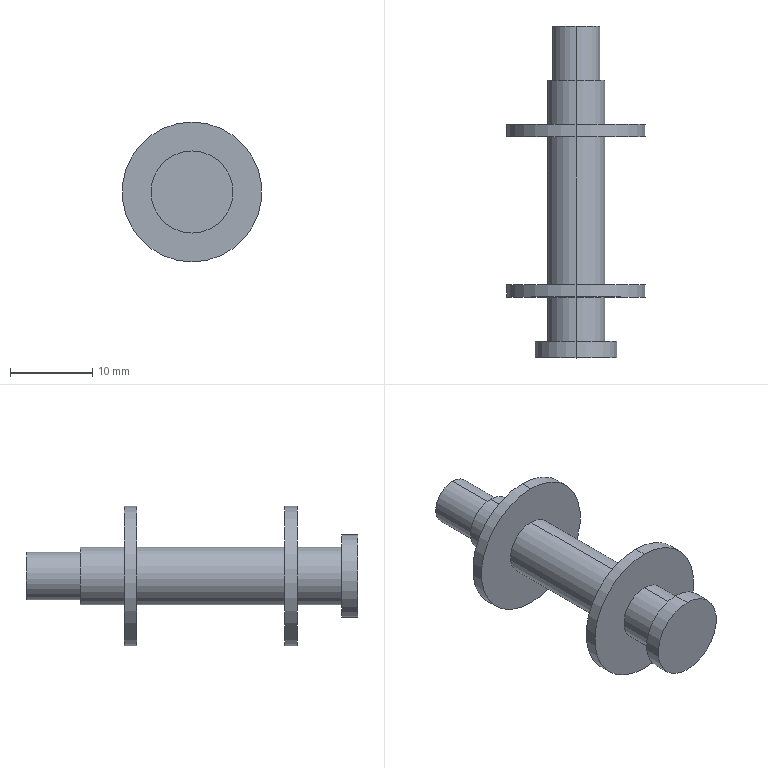Part | SolidWorks | features ICE 6, Extrusion 1 | 1 solid | 22 faces | box 17 x 40.37 x 17 mm | volume 2118 mm3 | cylinder 14 | plane 8 | commonest cylinder face diameters 7 x6 17 x4 5.77 x2 10 x2
STEP:
#1=CARTESIAN_POINT('',(0.,40.37,2.885));
#2=VERTEX_POINT('',#1);
#3=CARTESIAN_POINT('',(0.,40.37,-2.885));
#4=VERTEX_POINT('',#3);
#5=CARTESIAN_POINT('',(0.,40.37,0.));
#6=DIRECTION('',(0.,1.,0.));
#7=DIRECTION('',(0.,0.,1.));
#8=AXIS2_PLACEMENT_3D('',#5,#6,#7);
#9=CIRCLE('',#8,2.885);
#10=EDGE_CURVE('',#2,#4,#9,.T.);
#11=ORIENTED_EDGE('',*,*,#10,.F.);
#12=CARTESIAN_POINT('',(0.,33.8,2.885));
#13=VERTEX_POINT('',#12);
#14=CARTESIAN_POINT('',(0.,40.37,2.885));
#15=DIRECTION('',(0.,-1.,0.));
#16=VECTOR('',#15,1000.);
#17=LINE('',#14,#16);
#18=EDGE_CURVE('',#2,#13,#17,.T.);
#19=ORIENTED_EDGE('',*,*,#18,.T.);
#20=CARTESIAN_POINT('',(0.,33.8,-2.885));
#21=VERTEX_POINT('',#20);
#22=CARTESIAN_POINT('',(0.,33.8,0.));
#23=DIRECTION('',(0.,1.,0.));
#24=DIRECTION('',(0.,0.,1.));
#25=AXIS2_PLACEMENT_3D('',#22,#23,#24);
#26=CIRCLE('',#25,2.885);
#27=EDGE_CURVE('',#13,#21,#26,.T.);
#28=ORIENTED_EDGE('',*,*,#27,.T.);
#29=CARTESIAN_POINT('',(0.,40.37,-2.885));
#30=DIRECTION('',(0.,-1.,0.));
#31=VECTOR('',#30,1000.);
#32=LINE('',#29,#31);
#33=EDGE_CURVE('',#4,#21,#32,.T.);
#34=ORIENTED_EDGE('',*,*,#33,.F.);
#35=EDGE_LOOP('',(#11,#19,#28,#34));
#36=FACE_OUTER_BOUND('',#35,.T.);
#37=CARTESIAN_POINT('',(0.,40.37,0.));
#38=DIRECTION('',(0.,-1.,0.));
#39=DIRECTION('',(0.,0.,-1.));
#40=AXIS2_PLACEMENT_3D('',#37,#38,#39);
#41=CYLINDRICAL_SURFACE('',#40,2.885);
#42=ADVANCED_FACE('',(#36),#41,.T.);
#43=CARTESIAN_POINT('',(0.,33.8,3.5));
#44=VERTEX_POINT('',#43);
#45=CARTESIAN_POINT('',(0.,33.8,-3.5));
#46=VERTEX_POINT('',#45);
#47=CARTESIAN_POINT('',(0.,33.8,0.));
#48=DIRECTION('',(0.,1.,0.));
#49=DIRECTION('',(0.,0.,1.));
#50=AXIS2_PLACEMENT_3D('',#47,#48,#49);
#51=CIRCLE('',#50,3.5);
#52=EDGE_CURVE('',#44,#46,#51,.T.);
#53=ORIENTED_EDGE('',*,*,#52,.F.);
#54=CARTESIAN_POINT('',(0.,28.4,3.5));
#55=VERTEX_POINT('',#54);
#56=CARTESIAN_POINT('',(0.,33.8,3.5));
#57=DIRECTION('',(0.,-1.,0.));
#58=VECTOR('',#57,1000.);
#59=LINE('',#56,#58);
#60=EDGE_CURVE('',#44,#55,#59,.T.);
#61=ORIENTED_EDGE('',*,*,#60,.T.);
#62=CARTESIAN_POINT('',(0.,28.4,-3.5));
#63=VERTEX_POINT('',#62);
#64=CARTESIAN_POINT('',(0.,28.4,0.));
#65=DIRECTION('',(0.,1.,0.));
#66=DIRECTION('',(0.,0.,1.));
#67=AXIS2_PLACEMENT_3D('',#64,#65,#66);
#68=CIRCLE('',#67,3.5);
#69=EDGE_CURVE('',#55,#63,#68,.T.);
#70=ORIENTED_EDGE('',*,*,#69,.T.);
#71=CARTESIAN_POINT('',(0.,33.8,-3.5));
#72=DIRECTION('',(0.,-1.,0.));
#73=VECTOR('',#72,1000.);
#74=LINE('',#71,#73);
#75=EDGE_CURVE('',#46,#63,#74,.T.);
#76=ORIENTED_EDGE('',*,*,#75,.F.);
#77=EDGE_LOOP('',(#53,#61,#70,#76));
#78=FACE_OUTER_BOUND('',#77,.T.);
#79=CARTESIAN_POINT('',(0.,33.8,0.));
#80=DIRECTION('',(0.,-1.,0.));
#81=DIRECTION('',(0.,0.,-1.));
#82=AXIS2_PLACEMENT_3D('',#79,#80,#81);
#83=CYLINDRICAL_SURFACE('',#82,3.5);
#84=ADVANCED_FACE('',(#78),#83,.T.);
#85=CARTESIAN_POINT('',(0.,28.4,8.5));
#86=VERTEX_POINT('',#85);
#87=CARTESIAN_POINT('',(0.,28.4,-8.5));
#88=VERTEX_POINT('',#87);
#89=CARTESIAN_POINT('',(0.,28.4,0.));
#90=DIRECTION('',(0.,1.,0.));
#91=DIRECTION('',(0.,0.,1.));
#92=AXIS2_PLACEMENT_3D('',#89,#90,#91);
#93=CIRCLE('',#92,8.5);
#94=EDGE_CURVE('',#86,#88,#93,.T.);
#95=ORIENTED_EDGE('',*,*,#94,.F.);
#96=CARTESIAN_POINT('',(0.,26.9,8.5));
#97=VERTEX_POINT('',#96);
#98=CARTESIAN_POINT('',(0.,28.4,8.5));
#99=DIRECTION('',(0.,-1.,0.));
#100=VECTOR('',#99,1000.);
#101=LINE('',#98,#100);
#102=EDGE_CURVE('',#86,#97,#101,.T.);
#103=ORIENTED_EDGE('',*,*,#102,.T.);
#104=CARTESIAN_POINT('',(0.,26.9,-8.5));
#105=VERTEX_POINT('',#104);
#106=CARTESIAN_POINT('',(0.,26.9,0.));
#107=DIRECTION('',(0.,1.,0.));
#108=DIRECTION('',(0.,0.,1.));
#109=AXIS2_PLACEMENT_3D('',#106,#107,#108);
#110=CIRCLE('',#109,8.5);
#111=EDGE_CURVE('',#97,#105,#110,.T.);
#112=ORIENTED_EDGE('',*,*,#111,.T.);
#113=CARTESIAN_POINT('',(0.,28.4,-8.5));
#114=DIRECTION('',(0.,-1.,0.));
#115=VECTOR('',#114,1000.);
#116=LINE('',#113,#115);
#117=EDGE_CURVE('',#88,#105,#116,.T.);
#118=ORIENTED_EDGE('',*,*,#117,.F.);
#119=EDGE_LOOP('',(#95,#103,#112,#118));
#120=FACE_OUTER_BOUND('',#119,.T.);
#121=CARTESIAN_POINT('',(0.,28.4,0.));
#122=DIRECTION('',(0.,-1.,0.));
#123=DIRECTION('',(0.,0.,-1.));
#124=AXIS2_PLACEMENT_3D('',#121,#122,#123);
#125=CYLINDRICAL_SURFACE('',#124,8.5);
#126=ADVANCED_FACE('',(#120),#125,.T.);
#127=CARTESIAN_POINT('',(0.,26.9,3.5));
#128=VERTEX_POINT('',#127);
#129=CARTESIAN_POINT('',(0.,26.9,-3.5));
#130=VERTEX_POINT('',#129);
#131=CARTESIAN_POINT('',(0.,26.9,0.));
#132=DIRECTION('',(0.,1.,0.));
#133=DIRECTION('',(0.,0.,1.));
#134=AXIS2_PLACEMENT_3D('',#131,#132,#133);
#135=CIRCLE('',#134,3.5);
#136=EDGE_CURVE('',#128,#130,#135,.T.);
#137=ORIENTED_EDGE('',*,*,#136,.F.);
#138=CARTESIAN_POINT('',(0.,8.9,3.5));
#139=VERTEX_POINT('',#138);
#140=CARTESIAN_POINT('',(0.,26.9,3.5));
#141=DIRECTION('',(0.,-1.,0.));
#142=VECTOR('',#141,1000.);
#143=LINE('',#140,#142);
#144=EDGE_CURVE('',#128,#139,#143,.T.);
#145=ORIENTED_EDGE('',*,*,#144,.T.);
#146=CARTESIAN_POINT('',(0.,8.9,-3.5));
#147=VERTEX_POINT('',#146);
#148=CARTESIAN_POINT('',(0.,8.9,0.));
#149=DIRECTION('',(0.,1.,0.));
#150=DIRECTION('',(0.,0.,1.));
#151=AXIS2_PLACEMENT_3D('',#148,#149,#150);
#152=CIRCLE('',#151,3.5);
#153=EDGE_CURVE('',#139,#147,#152,.T.);
#154=ORIENTED_EDGE('',*,*,#153,.T.);
#155=CARTESIAN_POINT('',(0.,26.9,-3.5));
#156=DIRECTION('',(0.,-1.,0.));
#157=VECTOR('',#156,1000.);
#158=LINE('',#155,#157);
#159=EDGE_CURVE('',#130,#147,#158,.T.);
#160=ORIENTED_EDGE('',*,*,#159,.F.);
#161=EDGE_LOOP('',(#137,#145,#154,#160));
#162=FACE_OUTER_BOUND('',#161,.T.);
#163=CARTESIAN_POINT('',(0.,26.9,0.));
#164=DIRECTION('',(0.,-1.,0.));
#165=DIRECTION('',(0.,0.,-1.));
#166=AXIS2_PLACEMENT_3D('',#163,#164,#165);
#167=CYLINDRICAL_SURFACE('',#166,3.5);
#168=ADVANCED_FACE('',(#162),#167,.T.);
#169=CARTESIAN_POINT('',(0.,8.9,8.5));
#170=VERTEX_POINT('',#169);
#171=CARTESIAN_POINT('',(0.,8.9,-8.5));
#172=VERTEX_POINT('',#171);
#173=CARTESIAN_POINT('',(0.,8.9,0.));
#174=DIRECTION('',(0.,1.,0.));
#175=DIRECTION('',(0.,0.,1.));
#176=AXIS2_PLACEMENT_3D('',#173,#174,#175);
#177=CIRCLE('',#176,8.5);
#178=EDGE_CURVE('',#170,#172,#177,.T.);
#179=ORIENTED_EDGE('',*,*,#178,.F.);
#180=CARTESIAN_POINT('',(0.,7.4,8.5));
#181=VERTEX_POINT('',#180);
#182=CARTESIAN_POINT('',(0.,8.9,8.5));
#183=DIRECTION('',(0.,-1.,0.));
#184=VECTOR('',#183,1000.);
#185=LINE('',#182,#184);
#186=EDGE_CURVE('',#170,#181,#185,.T.);
#187=ORIENTED_EDGE('',*,*,#186,.T.);
#188=CARTESIAN_POINT('',(0.,7.4,-8.5));
#189=VERTEX_POINT('',#188);
#190=CARTESIAN_POINT('',(0.,7.4,0.));
#191=DIRECTION('',(0.,1.,0.));
#192=DIRECTION('',(0.,0.,1.));
#193=AXIS2_PLACEMENT_3D('',#190,#191,#192);
#194=CIRCLE('',#193,8.5);
#195=EDGE_CURVE('',#181,#189,#194,.T.);
#196=ORIENTED_EDGE('',*,*,#195,.T.);
#197=CARTESIAN_POINT('',(0.,8.9,-8.5));
#198=DIRECTION('',(0.,-1.,0.));
#199=VECTOR('',#198,1000.);
#200=LINE('',#197,#199);
#201=EDGE_CURVE('',#172,#189,#200,.T.);
#202=ORIENTED_EDGE('',*,*,#201,.F.);
#203=EDGE_LOOP('',(#179,#187,#196,#202));
#204=FACE_OUTER_BOUND('',#203,.T.);
#205=CARTESIAN_POINT('',(0.,8.9,0.));
#206=DIRECTION('',(0.,-1.,0.));
#207=DIRECTION('',(0.,0.,-1.));
#208=AXIS2_PLACEMENT_3D('',#205,#206,#207);
#209=CYLINDRICAL_SURFACE('',#208,8.5);
#210=ADVANCED_FACE('',(#204),#209,.T.);
#211=CARTESIAN_POINT('',(0.,7.4,3.5));
#212=VERTEX_POINT('',#211);
#213=CARTESIAN_POINT('',(0.,7.4,-3.5));
#214=VERTEX_POINT('',#213);
#215=CARTESIAN_POINT('',(0.,7.4,0.));
#216=DIRECTION('',(0.,1.,0.));
#217=DIRECTION('',(0.,0.,1.));
#218=AXIS2_PLACEMENT_3D('',#215,#216,#217);
#219=CIRCLE('',#218,3.5);
#220=EDGE_CURVE('',#212,#214,#219,.T.);
#221=ORIENTED_EDGE('',*,*,#220,.F.);
#222=CARTESIAN_POINT('',(0.,2.,3.5));
#223=VERTEX_POINT('',#222);
#224=CARTESIAN_POINT('',(0.,7.4,3.5));
#225=DIRECTION('',(0.,-1.,0.));
#226=VECTOR('',#225,1000.);
#227=LINE('',#224,#226);
#228=EDGE_CURVE('',#212,#223,#227,.T.);
#229=ORIENTED_EDGE('',*,*,#228,.T.);
#230=CARTESIAN_POINT('',(0.,2.,-3.5));
#231=VERTEX_POINT('',#230);
#232=CARTESIAN_POINT('',(0.,2.,0.));
#233=DIRECTION('',(0.,1.,0.));
#234=DIRECTION('',(0.,0.,1.));
#235=AXIS2_PLACEMENT_3D('',#232,#233,#234);
#236=CIRCLE('',#235,3.5);
#237=EDGE_CURVE('',#223,#231,#236,.T.);
#238=ORIENTED_EDGE('',*,*,#237,.T.);
#239=CARTESIAN_POINT('',(0.,7.4,-3.5));
#240=DIRECTION('',(0.,-1.,0.));
#241=VECTOR('',#240,1000.);
#242=LINE('',#239,#241);
#243=EDGE_CURVE('',#214,#231,#242,.T.);
#244=ORIENTED_EDGE('',*,*,#243,.F.);
#245=EDGE_LOOP('',(#221,#229,#238,#244));
#246=FACE_OUTER_BOUND('',#245,.T.);
#247=CARTESIAN_POINT('',(0.,7.4,0.));
#248=DIRECTION('',(0.,-1.,0.));
#249=DIRECTION('',(0.,0.,-1.));
#250=AXIS2_PLACEMENT_3D('',#247,#248,#249);
#251=CYLINDRICAL_SURFACE('',#250,3.5);
#252=ADVANCED_FACE('',(#246),#251,.T.);
#253=CARTESIAN_POINT('',(0.,2.,5.));
#254=VERTEX_POINT('',#253);
#255=CARTESIAN_POINT('',(0.,2.,-5.));
#256=VERTEX_POINT('',#255);
#257=CARTESIAN_POINT('',(0.,2.,0.));
#258=DIRECTION('',(0.,1.,0.));
#259=DIRECTION('',(0.,0.,1.));
#260=AXIS2_PLACEMENT_3D('',#257,#258,#259);
#261=CIRCLE('',#260,5.);
#262=EDGE_CURVE('',#254,#256,#261,.T.);
#263=ORIENTED_EDGE('',*,*,#262,.F.);
#264=CARTESIAN_POINT('',(0.,0.,5.));
#265=VERTEX_POINT('',#264);
#266=CARTESIAN_POINT('',(0.,2.,5.));
#267=DIRECTION('',(0.,-1.,0.));
#268=VECTOR('',#267,1000.);
#269=LINE('',#266,#268);
#270=EDGE_CURVE('',#254,#265,#269,.T.);
#271=ORIENTED_EDGE('',*,*,#270,.T.);
#272=CARTESIAN_POINT('',(0.,0.,-5.));
#273=VERTEX_POINT('',#272);
#274=CARTESIAN_POINT('',(0.,0.,0.));
#275=DIRECTION('',(0.,1.,0.));
#276=DIRECTION('',(0.,0.,1.));
#277=AXIS2_PLACEMENT_3D('',#274,#275,#276);
#278=CIRCLE('',#277,5.);
#279=EDGE_CURVE('',#265,#273,#278,.T.);
#280=ORIENTED_EDGE('',*,*,#279,.T.);
#281=CARTESIAN_POINT('',(0.,2.,-5.));
#282=DIRECTION('',(0.,-1.,0.));
#283=VECTOR('',#282,1000.);
#284=LINE('',#281,#283);
#285=EDGE_CURVE('',#256,#273,#284,.T.);
#286=ORIENTED_EDGE('',*,*,#285,.F.);
#287=EDGE_LOOP('',(#263,#271,#280,#286));
#288=FACE_OUTER_BOUND('',#287,.T.);
#289=CARTESIAN_POINT('',(0.,2.,0.));
#290=DIRECTION('',(0.,-1.,0.));
#291=DIRECTION('',(0.,0.,-1.));
#292=AXIS2_PLACEMENT_3D('',#289,#290,#291);
#293=CYLINDRICAL_SURFACE('',#292,5.);
#294=ADVANCED_FACE('',(#288),#293,.T.);
#295=ORIENTED_EDGE('',*,*,#270,.F.);
#296=CARTESIAN_POINT('',(0.,2.,0.));
#297=DIRECTION('',(0.,1.,0.));
#298=DIRECTION('',(0.,0.,1.));
#299=AXIS2_PLACEMENT_3D('',#296,#297,#298);
#300=CIRCLE('',#299,5.);
#301=EDGE_CURVE('',#256,#254,#300,.T.);
#302=ORIENTED_EDGE('',*,*,#301,.F.);
#303=ORIENTED_EDGE('',*,*,#285,.T.);
#304=CARTESIAN_POINT('',(0.,0.,0.));
#305=DIRECTION('',(0.,1.,0.));
#306=DIRECTION('',(0.,0.,1.));
#307=AXIS2_PLACEMENT_3D('',#304,#305,#306);
#308=CIRCLE('',#307,5.);
#309=EDGE_CURVE('',#273,#265,#308,.T.);
#310=ORIENTED_EDGE('',*,*,#309,.T.);
#311=EDGE_LOOP('',(#295,#302,#303,#310));
#312=FACE_OUTER_BOUND('',#311,.T.);
#313=CARTESIAN_POINT('',(0.,2.,0.));
#314=DIRECTION('',(0.,-1.,0.));
#315=DIRECTION('',(0.,0.,-1.));
#316=AXIS2_PLACEMENT_3D('',#313,#314,#315);
#317=CYLINDRICAL_SURFACE('',#316,5.);
#318=ADVANCED_FACE('',(#312),#317,.T.);
#319=CARTESIAN_POINT('',(0.,2.,0.));
#320=DIRECTION('',(0.,1.,0.));
#321=DIRECTION('',(0.,0.,1.));
#322=AXIS2_PLACEMENT_3D('',#319,#320,#321);
#323=CIRCLE('',#322,3.5);
#324=EDGE_CURVE('',#231,#223,#323,.T.);
#325=ORIENTED_EDGE('',*,*,#324,.F.);
#326=ORIENTED_EDGE('',*,*,#237,.F.);
#327=EDGE_LOOP('',(#325,#326));
#328=FACE_BOUND('',#327,.T.);
#329=ORIENTED_EDGE('',*,*,#301,.T.);
#330=ORIENTED_EDGE('',*,*,#262,.T.);
#331=EDGE_LOOP('',(#329,#330));
#332=FACE_OUTER_BOUND('',#331,.T.);
#333=CARTESIAN_POINT('',(0.,2.,0.));
#334=DIRECTION('',(0.,1.,0.));
#335=DIRECTION('',(0.,0.,1.));
#336=AXIS2_PLACEMENT_3D('',#333,#334,#335);
#337=PLANE('',#336);
#338=ADVANCED_FACE('',(#328,#332),#337,.T.);
#339=ORIENTED_EDGE('',*,*,#309,.F.);
#340=ORIENTED_EDGE('',*,*,#279,.F.);
#341=EDGE_LOOP('',(#339,#340));
#342=FACE_OUTER_BOUND('',#341,.T.);
#343=CARTESIAN_POINT('',(0.,0.,0.));
#344=DIRECTION('',(0.,1.,0.));
#345=DIRECTION('',(0.,0.,1.));
#346=AXIS2_PLACEMENT_3D('',#343,#344,#345);
#347=PLANE('',#346);
#348=ADVANCED_FACE('',(#342),#347,.F.);
#349=ORIENTED_EDGE('',*,*,#228,.F.);
#350=CARTESIAN_POINT('',(0.,7.4,0.));
#351=DIRECTION('',(0.,1.,0.));
#352=DIRECTION('',(0.,0.,1.));
#353=AXIS2_PLACEMENT_3D('',#350,#351,#352);
#354=CIRCLE('',#353,3.5);
#355=EDGE_CURVE('',#214,#212,#354,.T.);
#356=ORIENTED_EDGE('',*,*,#355,.F.);
#357=ORIENTED_EDGE('',*,*,#243,.T.);
#358=ORIENTED_EDGE('',*,*,#324,.T.);
#359=EDGE_LOOP('',(#349,#356,#357,#358));
#360=FACE_OUTER_BOUND('',#359,.T.);
#361=CARTESIAN_POINT('',(0.,7.4,0.));
#362=DIRECTION('',(0.,-1.,0.));
#363=DIRECTION('',(0.,0.,-1.));
#364=AXIS2_PLACEMENT_3D('',#361,#362,#363);
#365=CYLINDRICAL_SURFACE('',#364,3.5);
#366=ADVANCED_FACE('',(#360),#365,.T.);
#367=ORIENTED_EDGE('',*,*,#186,.F.);
#368=CARTESIAN_POINT('',(0.,8.9,0.));
#369=DIRECTION('',(0.,1.,0.));
#370=DIRECTION('',(0.,0.,1.));
#371=AXIS2_PLACEMENT_3D('',#368,#369,#370);
#372=CIRCLE('',#371,8.5);
#373=EDGE_CURVE('',#172,#170,#372,.T.);
#374=ORIENTED_EDGE('',*,*,#373,.F.);
#375=ORIENTED_EDGE('',*,*,#201,.T.);
#376=CARTESIAN_POINT('',(0.,7.4,0.));
#377=DIRECTION('',(0.,1.,0.));
#378=DIRECTION('',(0.,0.,1.));
#379=AXIS2_PLACEMENT_3D('',#376,#377,#378);
#380=CIRCLE('',#379,8.5);
#381=EDGE_CURVE('',#189,#181,#380,.T.);
#382=ORIENTED_EDGE('',*,*,#381,.T.);
#383=EDGE_LOOP('',(#367,#374,#375,#382));
#384=FACE_OUTER_BOUND('',#383,.T.);
#385=CARTESIAN_POINT('',(0.,8.9,0.));
#386=DIRECTION('',(0.,-1.,0.));
#387=DIRECTION('',(0.,0.,-1.));
#388=AXIS2_PLACEMENT_3D('',#385,#386,#387);
#389=CYLINDRICAL_SURFACE('',#388,8.5);
#390=ADVANCED_FACE('',(#384),#389,.T.);
#391=CARTESIAN_POINT('',(0.,8.9,0.));
#392=DIRECTION('',(0.,1.,0.));
#393=DIRECTION('',(0.,0.,1.));
#394=AXIS2_PLACEMENT_3D('',#391,#392,#393);
#395=CIRCLE('',#394,3.5);
#396=EDGE_CURVE('',#147,#139,#395,.T.);
#397=ORIENTED_EDGE('',*,*,#396,.F.);
#398=ORIENTED_EDGE('',*,*,#153,.F.);
#399=EDGE_LOOP('',(#397,#398));
#400=FACE_BOUND('',#399,.T.);
#401=ORIENTED_EDGE('',*,*,#373,.T.);
#402=ORIENTED_EDGE('',*,*,#178,.T.);
#403=EDGE_LOOP('',(#401,#402));
#404=FACE_OUTER_BOUND('',#403,.T.);
#405=CARTESIAN_POINT('',(0.,8.9,0.));
#406=DIRECTION('',(0.,1.,0.));
#407=DIRECTION('',(0.,0.,1.));
#408=AXIS2_PLACEMENT_3D('',#405,#406,#407);
#409=PLANE('',#408);
#410=ADVANCED_FACE('',(#400,#404),#409,.T.);
#411=ORIENTED_EDGE('',*,*,#355,.T.);
#412=ORIENTED_EDGE('',*,*,#220,.T.);
#413=EDGE_LOOP('',(#411,#412));
#414=FACE_BOUND('',#413,.T.);
#415=ORIENTED_EDGE('',*,*,#381,.F.);
#416=ORIENTED_EDGE('',*,*,#195,.F.);
#417=EDGE_LOOP('',(#415,#416));
#418=FACE_OUTER_BOUND('',#417,.T.);
#419=CARTESIAN_POINT('',(0.,7.4,0.));
#420=DIRECTION('',(0.,1.,0.));
#421=DIRECTION('',(0.,0.,1.));
#422=AXIS2_PLACEMENT_3D('',#419,#420,#421);
#423=PLANE('',#422);
#424=ADVANCED_FACE('',(#414,#418),#423,.F.);
#425=ORIENTED_EDGE('',*,*,#144,.F.);
#426=CARTESIAN_POINT('',(0.,26.9,0.));
#427=DIRECTION('',(0.,1.,0.));
#428=DIRECTION('',(0.,0.,1.));
#429=AXIS2_PLACEMENT_3D('',#426,#427,#428);
#430=CIRCLE('',#429,3.5);
#431=EDGE_CURVE('',#130,#128,#430,.T.);
#432=ORIENTED_EDGE('',*,*,#431,.F.);
#433=ORIENTED_EDGE('',*,*,#159,.T.);
#434=ORIENTED_EDGE('',*,*,#396,.T.);
#435=EDGE_LOOP('',(#425,#432,#433,#434));
#436=FACE_OUTER_BOUND('',#435,.T.);
#437=CARTESIAN_POINT('',(0.,26.9,0.));
#438=DIRECTION('',(0.,-1.,0.));
#439=DIRECTION('',(0.,0.,-1.));
#440=AXIS2_PLACEMENT_3D('',#437,#438,#439);
#441=CYLINDRICAL_SURFACE('',#440,3.5);
#442=ADVANCED_FACE('',(#436),#441,.T.);
#443=ORIENTED_EDGE('',*,*,#102,.F.);
#444=CARTESIAN_POINT('',(0.,28.4,0.));
#445=DIRECTION('',(0.,1.,0.));
#446=DIRECTION('',(0.,0.,1.));
#447=AXIS2_PLACEMENT_3D('',#444,#445,#446);
#448=CIRCLE('',#447,8.5);
#449=EDGE_CURVE('',#88,#86,#448,.T.);
#450=ORIENTED_EDGE('',*,*,#449,.F.);
#451=ORIENTED_EDGE('',*,*,#117,.T.);
#452=CARTESIAN_POINT('',(0.,26.9,0.));
#453=DIRECTION('',(0.,1.,0.));
#454=DIRECTION('',(0.,0.,1.));
#455=AXIS2_PLACEMENT_3D('',#452,#453,#454);
#456=CIRCLE('',#455,8.5);
#457=EDGE_CURVE('',#105,#97,#456,.T.);
#458=ORIENTED_EDGE('',*,*,#457,.T.);
#459=EDGE_LOOP('',(#443,#450,#451,#458));
#460=FACE_OUTER_BOUND('',#459,.T.);
#461=CARTESIAN_POINT('',(0.,28.4,0.));
#462=DIRECTION('',(0.,-1.,0.));
#463=DIRECTION('',(0.,0.,-1.));
#464=AXIS2_PLACEMENT_3D('',#461,#462,#463);
#465=CYLINDRICAL_SURFACE('',#464,8.5);
#466=ADVANCED_FACE('',(#460),#465,.T.);
#467=CARTESIAN_POINT('',(0.,28.4,0.));
#468=DIRECTION('',(0.,1.,0.));
#469=DIRECTION('',(0.,0.,1.));
#470=AXIS2_PLACEMENT_3D('',#467,#468,#469);
#471=CIRCLE('',#470,3.5);
#472=EDGE_CURVE('',#63,#55,#471,.T.);
#473=ORIENTED_EDGE('',*,*,#472,.F.);
#474=ORIENTED_EDGE('',*,*,#69,.F.);
#475=EDGE_LOOP('',(#473,#474));
#476=FACE_BOUND('',#475,.T.);
#477=ORIENTED_EDGE('',*,*,#449,.T.);
#478=ORIENTED_EDGE('',*,*,#94,.T.);
#479=EDGE_LOOP('',(#477,#478));
#480=FACE_OUTER_BOUND('',#479,.T.);
#481=CARTESIAN_POINT('',(0.,28.4,0.));
#482=DIRECTION('',(0.,1.,0.));
#483=DIRECTION('',(0.,0.,1.));
#484=AXIS2_PLACEMENT_3D('',#481,#482,#483);
#485=PLANE('',#484);
#486=ADVANCED_FACE('',(#476,#480),#485,.T.);
#487=ORIENTED_EDGE('',*,*,#431,.T.);
#488=ORIENTED_EDGE('',*,*,#136,.T.);
#489=EDGE_LOOP('',(#487,#488));
#490=FACE_BOUND('',#489,.T.);
#491=ORIENTED_EDGE('',*,*,#457,.F.);
#492=ORIENTED_EDGE('',*,*,#111,.F.);
#493=EDGE_LOOP('',(#491,#492));
#494=FACE_OUTER_BOUND('',#493,.T.);
#495=CARTESIAN_POINT('',(0.,26.9,0.));
#496=DIRECTION('',(0.,1.,0.));
#497=DIRECTION('',(0.,0.,1.));
#498=AXIS2_PLACEMENT_3D('',#495,#496,#497);
#499=PLANE('',#498);
#500=ADVANCED_FACE('',(#490,#494),#499,.F.);
#501=ORIENTED_EDGE('',*,*,#60,.F.);
#502=CARTESIAN_POINT('',(0.,33.8,0.));
#503=DIRECTION('',(0.,1.,0.));
#504=DIRECTION('',(0.,0.,1.));
#505=AXIS2_PLACEMENT_3D('',#502,#503,#504);
#506=CIRCLE('',#505,3.5);
#507=EDGE_CURVE('',#46,#44,#506,.T.);
#508=ORIENTED_EDGE('',*,*,#507,.F.);
#509=ORIENTED_EDGE('',*,*,#75,.T.);
#510=ORIENTED_EDGE('',*,*,#472,.T.);
#511=EDGE_LOOP('',(#501,#508,#509,#510));
#512=FACE_OUTER_BOUND('',#511,.T.);
#513=CARTESIAN_POINT('',(0.,33.8,0.));
#514=DIRECTION('',(0.,-1.,0.));
#515=DIRECTION('',(0.,0.,-1.));
#516=AXIS2_PLACEMENT_3D('',#513,#514,#515);
#517=CYLINDRICAL_SURFACE('',#516,3.5);
#518=ADVANCED_FACE('',(#512),#517,.T.);
#519=CARTESIAN_POINT('',(0.,33.8,0.));
#520=DIRECTION('',(0.,1.,0.));
#521=DIRECTION('',(0.,0.,1.));
#522=AXIS2_PLACEMENT_3D('',#519,#520,#521);
#523=CIRCLE('',#522,2.885);
#524=EDGE_CURVE('',#21,#13,#523,.T.);
#525=ORIENTED_EDGE('',*,*,#524,.F.);
#526=ORIENTED_EDGE('',*,*,#27,.F.);
#527=EDGE_LOOP('',(#525,#526));
#528=FACE_BOUND('',#527,.T.);
#529=ORIENTED_EDGE('',*,*,#507,.T.);
#530=ORIENTED_EDGE('',*,*,#52,.T.);
#531=EDGE_LOOP('',(#529,#530));
#532=FACE_OUTER_BOUND('',#531,.T.);
#533=CARTESIAN_POINT('',(0.,33.8,0.));
#534=DIRECTION('',(0.,1.,0.));
#535=DIRECTION('',(0.,0.,1.));
#536=AXIS2_PLACEMENT_3D('',#533,#534,#535);
#537=PLANE('',#536);
#538=ADVANCED_FACE('',(#528,#532),#537,.T.);
#539=ORIENTED_EDGE('',*,*,#18,.F.);
#540=CARTESIAN_POINT('',(0.,40.37,0.));
#541=DIRECTION('',(0.,1.,0.));
#542=DIRECTION('',(0.,0.,1.));
#543=AXIS2_PLACEMENT_3D('',#540,#541,#542);
#544=CIRCLE('',#543,2.885);
#545=EDGE_CURVE('',#4,#2,#544,.T.);
#546=ORIENTED_EDGE('',*,*,#545,.F.);
#547=ORIENTED_EDGE('',*,*,#33,.T.);
#548=ORIENTED_EDGE('',*,*,#524,.T.);
#549=EDGE_LOOP('',(#539,#546,#547,#548));
#550=FACE_OUTER_BOUND('',#549,.T.);
#551=CARTESIAN_POINT('',(0.,40.37,0.));
#552=DIRECTION('',(0.,-1.,0.));
#553=DIRECTION('',(0.,0.,-1.));
#554=AXIS2_PLACEMENT_3D('',#551,#552,#553);
#555=CYLINDRICAL_SURFACE('',#554,2.885);
#556=ADVANCED_FACE('',(#550),#555,.T.);
#557=ORIENTED_EDGE('',*,*,#545,.T.);
#558=ORIENTED_EDGE('',*,*,#10,.T.);
#559=EDGE_LOOP('',(#557,#558));
#560=FACE_OUTER_BOUND('',#559,.T.);
#561=CARTESIAN_POINT('',(0.,40.37,0.));
#562=DIRECTION('',(0.,1.,0.));
#563=DIRECTION('',(0.,0.,1.));
#564=AXIS2_PLACEMENT_3D('',#561,#562,#563);
#565=PLANE('',#564);
#566=ADVANCED_FACE('',(#560),#565,.T.);
#567=CLOSED_SHELL('',(#42,#84,#126,#168,#210,#252,#294,#318,#338,#348,#366,#390,#410,#424,#442,#466,#486,#500,#518,#538,#556,#566));
#568=MANIFOLD_SOLID_BREP('',#567);
#569=CARTESIAN_POINT('',(0.,0.,0.));
#570=DIRECTION('',(0.,0.,1.));
#571=DIRECTION('',(1.,0.,0.));
#572=AXIS2_PLACEMENT_3D('',#569,#570,#571);
#573=(LENGTH_UNIT()NAMED_UNIT(*)SI_UNIT(.MILLI.,.METRE.));
#574=UNCERTAINTY_MEASURE_WITH_UNIT(LENGTH_MEASURE(0.00001),#573,'','');
#575=(NAMED_UNIT(*)PLANE_ANGLE_UNIT()SI_UNIT($,.RADIAN.));
#576=(NAMED_UNIT(*)SI_UNIT($,.STERADIAN.)SOLID_ANGLE_UNIT());
#577=(GEOMETRIC_REPRESENTATION_CONTEXT(3)GLOBAL_UNCERTAINTY_ASSIGNED_CONTEXT((#574))GLOBAL_UNIT_ASSIGNED_CONTEXT((#573,#575,#576))REPRESENTATION_CONTEXT('',''));
#578=ADVANCED_BREP_SHAPE_REPRESENTATION('',(#568,#572),#577);